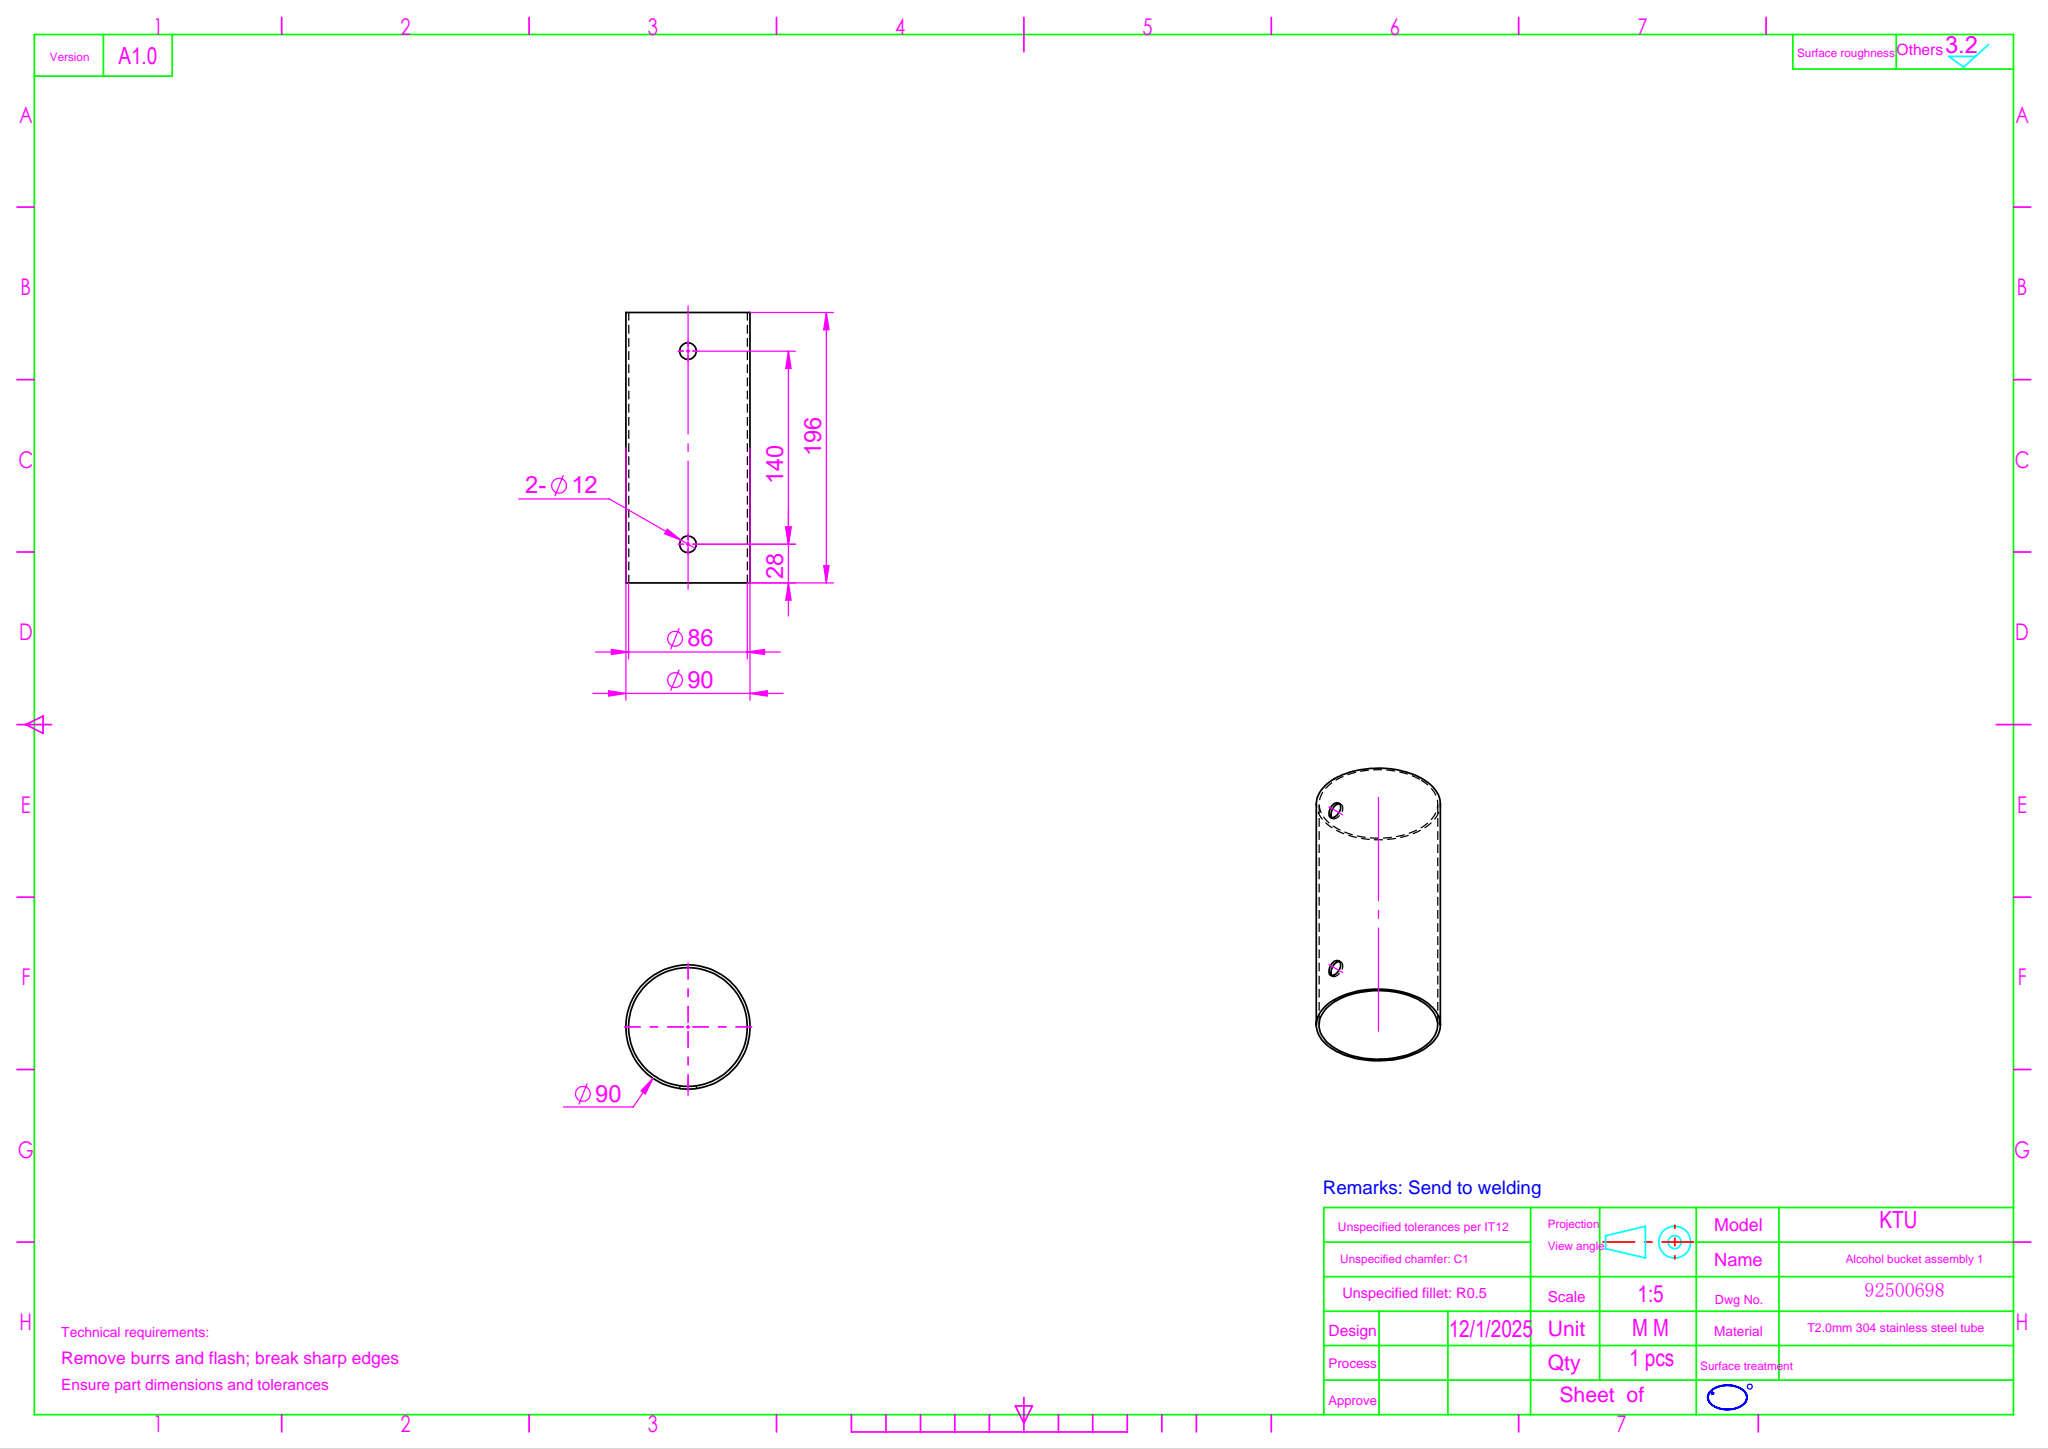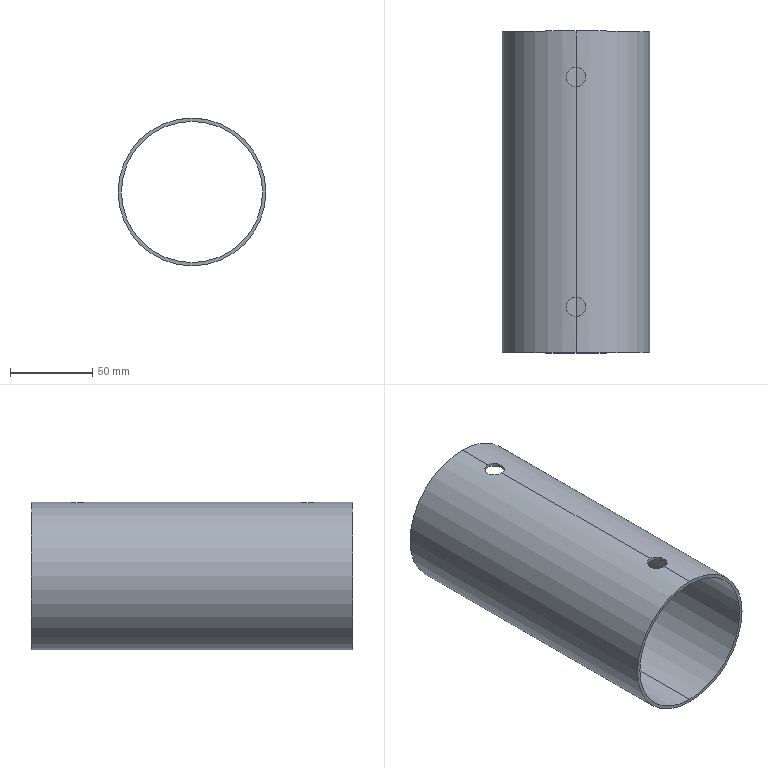Part | SolidWorks | features ExtruThin 1, ICE 1 | 1 solid | 10 faces | box 90 x 196 x 90 mm | volume 107919 mm3 | cylinder 8 | plane 2 | commonest cylinder face diameters 12 x4 86 x2 90 x2
STEP:
#1=CARTESIAN_POINT('',(0.,-76.,45.));
#2=VERTEX_POINT('',#1);
#3=CARTESIAN_POINT('',(6.,-70.,44.598));
#4=VERTEX_POINT('',#3);
#5=CARTESIAN_POINT('',(0.,-76.,45.));
#6=CARTESIAN_POINT('',(0.397,-76.,45.));
#7=CARTESIAN_POINT('',(0.7873,-75.961,44.995));
#8=CARTESIAN_POINT('',(1.363,-75.846,44.98));
#9=CARTESIAN_POINT('',(1.553,-75.799,44.974));
#10=CARTESIAN_POINT('',(1.931,-75.684,44.959));
#11=CARTESIAN_POINT('',(2.118,-75.617,44.95));
#12=CARTESIAN_POINT('',(2.663,-75.391,44.923));
#13=CARTESIAN_POINT('',(3.008,-75.207,44.901));
#14=CARTESIAN_POINT('',(3.66,-74.771,44.852));
#15=CARTESIAN_POINT('',(3.968,-74.518,44.826));
#16=CARTESIAN_POINT('',(4.521,-73.964,44.773));
#17=CARTESIAN_POINT('',(4.769,-73.662,44.747));
#18=CARTESIAN_POINT('',(5.098,-73.17,44.71));
#19=CARTESIAN_POINT('',(5.2,-73.,44.699));
#20=CARTESIAN_POINT('',(5.385,-72.654,44.677));
#21=CARTESIAN_POINT('',(5.552,-72.3,44.656));
#22=CARTESIAN_POINT('',(5.684,-71.932,44.64));
#23=CARTESIAN_POINT('',(5.798,-71.556,44.625));
#24=CARTESIAN_POINT('',(5.846,-71.363,44.619));
#25=CARTESIAN_POINT('',(5.962,-70.782,44.603));
#26=CARTESIAN_POINT('',(6.,-70.392,44.598));
#27=CARTESIAN_POINT('',(6.,-70.,44.598));
#28=B_SPLINE_CURVE_WITH_KNOTS('',3,(#5,#6,#7,#8,#9,#10,#11,#12,#13,#14,#15,#16,#17,#18,#19,#20,#21,#22,#23,#24,#25,#26,#27),.UNSPECIFIED.,.F.,.F.,(4,2,2,2,2,2,2,2,1,2,2,4),(0.,0.001174,0.001761,0.002348,0.003522,0.004696,0.00587,0.006457,0.007044,0.007631,0.008218,0.009392),.UNSPECIFIED.);
#29=EDGE_CURVE('',#2,#4,#28,.T.);
#30=ORIENTED_EDGE('',*,*,#29,.T.);
#31=CARTESIAN_POINT('',(6.,-70.,42.579));
#32=VERTEX_POINT('',#31);
#33=CARTESIAN_POINT('',(6.,-70.,45.));
#34=DIRECTION('',(0.,0.,-1.));
#35=VECTOR('',#34,1000.);
#36=LINE('',#33,#35);
#37=EDGE_CURVE('',#4,#32,#36,.T.);
#38=ORIENTED_EDGE('',*,*,#37,.T.);
#39=CARTESIAN_POINT('',(0.,-76.,43.));
#40=VERTEX_POINT('',#39);
#41=CARTESIAN_POINT('',(0.,-76.,43.));
#42=CARTESIAN_POINT('',(0.3918,-76.,43.));
#43=CARTESIAN_POINT('',(0.7898,-75.961,42.994));
#44=CARTESIAN_POINT('',(1.559,-75.807,42.973));
#45=CARTESIAN_POINT('',(1.934,-75.693,42.958));
#46=CARTESIAN_POINT('',(2.479,-75.468,42.929));
#47=CARTESIAN_POINT('',(2.659,-75.382,42.918));
#48=CARTESIAN_POINT('',(3.005,-75.197,42.895));
#49=CARTESIAN_POINT('',(3.173,-75.096,42.883));
#50=CARTESIAN_POINT('',(3.66,-74.77,42.845));
#51=CARTESIAN_POINT('',(3.964,-74.522,42.818));
#52=CARTESIAN_POINT('',(4.523,-73.962,42.762));
#53=CARTESIAN_POINT('',(4.771,-73.66,42.735));
#54=CARTESIAN_POINT('',(5.096,-73.173,42.697));
#55=CARTESIAN_POINT('',(5.197,-73.005,42.685));
#56=CARTESIAN_POINT('',(5.383,-72.658,42.662));
#57=CARTESIAN_POINT('',(5.468,-72.478,42.651));
#58=CARTESIAN_POINT('',(5.694,-71.933,42.622));
#59=CARTESIAN_POINT('',(5.807,-71.559,42.606));
#60=CARTESIAN_POINT('',(5.961,-70.79,42.585));
#61=CARTESIAN_POINT('',(6.,-70.392,42.579));
#62=CARTESIAN_POINT('',(6.,-70.,42.579));
#63=B_SPLINE_CURVE_WITH_KNOTS('',3,(#41,#42,#43,#44,#45,#46,#47,#48,#49,#50,#51,#52,#53,#54,#55,#56,#57,#58,#59,#60,#61,#62),.UNSPECIFIED.,.F.,.F.,(4,2,2,2,2,2,2,2,2,2,4),(0.009393,0.01057,0.01174,0.01233,0.01291,0.01409,0.01526,0.01585,0.01643,0.01761,0.01878),.UNSPECIFIED.);
#64=EDGE_CURVE('',#40,#32,#63,.T.);
#65=ORIENTED_EDGE('',*,*,#64,.F.);
#66=CARTESIAN_POINT('',(-6.,-70.,42.579));
#67=VERTEX_POINT('',#66);
#68=CARTESIAN_POINT('',(-6.,-70.,42.579));
#69=CARTESIAN_POINT('',(-6.,-70.397,42.579));
#70=CARTESIAN_POINT('',(-5.961,-70.787,42.585));
#71=CARTESIAN_POINT('',(-5.846,-71.363,42.601));
#72=CARTESIAN_POINT('',(-5.799,-71.553,42.607));
#73=CARTESIAN_POINT('',(-5.684,-71.931,42.623));
#74=CARTESIAN_POINT('',(-5.617,-72.118,42.632));
#75=CARTESIAN_POINT('',(-5.391,-72.663,42.661));
#76=CARTESIAN_POINT('',(-5.207,-73.008,42.684));
#77=CARTESIAN_POINT('',(-4.771,-73.66,42.735));
#78=CARTESIAN_POINT('',(-4.518,-73.968,42.763));
#79=CARTESIAN_POINT('',(-3.964,-74.521,42.818));
#80=CARTESIAN_POINT('',(-3.662,-74.769,42.845));
#81=CARTESIAN_POINT('',(-3.17,-75.098,42.883));
#82=CARTESIAN_POINT('',(-3.,-75.2,42.896));
#83=CARTESIAN_POINT('',(-2.654,-75.385,42.918));
#84=CARTESIAN_POINT('',(-2.3,-75.552,42.94));
#85=CARTESIAN_POINT('',(-1.932,-75.684,42.957));
#86=CARTESIAN_POINT('',(-1.556,-75.798,42.972));
#87=CARTESIAN_POINT('',(-1.363,-75.846,42.979));
#88=CARTESIAN_POINT('',(-0.7817,-75.962,42.995));
#89=CARTESIAN_POINT('',(-0.392,-76.,43.));
#90=CARTESIAN_POINT('',(0.,-76.,43.));
#91=B_SPLINE_CURVE_WITH_KNOTS('',3,(#68,#69,#70,#71,#72,#73,#74,#75,#76,#77,#78,#79,#80,#81,#82,#83,#84,#85,#86,#87,#88,#89,#90),.UNSPECIFIED.,.F.,.F.,(4,2,2,2,2,2,2,2,1,2,2,4),(0.,0.001174,0.001761,0.002348,0.003522,0.004697,0.005871,0.006458,0.007045,0.007632,0.008219,0.009393),.UNSPECIFIED.);
#92=EDGE_CURVE('',#67,#40,#91,.T.);
#93=ORIENTED_EDGE('',*,*,#92,.F.);
#94=CARTESIAN_POINT('',(-6.,-70.,44.598));
#95=VERTEX_POINT('',#94);
#96=CARTESIAN_POINT('',(-6.,-70.,45.));
#97=DIRECTION('',(0.,0.,-1.));
#98=VECTOR('',#97,1000.);
#99=LINE('',#96,#98);
#100=EDGE_CURVE('',#95,#67,#99,.T.);
#101=ORIENTED_EDGE('',*,*,#100,.F.);
#102=CARTESIAN_POINT('',(-6.,-70.,44.598));
#103=CARTESIAN_POINT('',(-6.,-70.396,44.598));
#104=CARTESIAN_POINT('',(-5.961,-70.786,44.603));
#105=CARTESIAN_POINT('',(-5.847,-71.362,44.619));
#106=CARTESIAN_POINT('',(-5.799,-71.552,44.625));
#107=CARTESIAN_POINT('',(-5.685,-71.929,44.64));
#108=CARTESIAN_POINT('',(-5.618,-72.116,44.648));
#109=CARTESIAN_POINT('',(-5.392,-72.661,44.676));
#110=CARTESIAN_POINT('',(-5.208,-73.005,44.698));
#111=CARTESIAN_POINT('',(-4.773,-73.657,44.747));
#112=CARTESIAN_POINT('',(-4.52,-73.965,44.773));
#113=CARTESIAN_POINT('',(-3.968,-74.517,44.826));
#114=CARTESIAN_POINT('',(-3.666,-74.766,44.852));
#115=CARTESIAN_POINT('',(-3.011,-75.205,44.9));
#116=CARTESIAN_POINT('',(-2.663,-75.391,44.923));
#117=CARTESIAN_POINT('',(-1.942,-75.69,44.96));
#118=CARTESIAN_POINT('',(-1.564,-75.806,44.974));
#119=CARTESIAN_POINT('',(-0.7887,-75.961,44.995));
#120=CARTESIAN_POINT('',(-0.3966,-76.,45.));
#121=CARTESIAN_POINT('',(0.,-76.,45.));
#122=B_SPLINE_CURVE_WITH_KNOTS('',3,(#102,#103,#104,#105,#106,#107,#108,#109,#110,#111,#112,#113,#114,#115,#116,#117,#118,#119,#120,#121),.UNSPECIFIED.,.F.,.F.,(4,2,2,2,2,2,2,2,2,4),(0.02817,0.02934,0.02993,0.03052,0.03169,0.03286,0.03404,0.03521,0.03638,0.03755),.UNSPECIFIED.);
#123=EDGE_CURVE('',#95,#2,#122,.T.);
#124=ORIENTED_EDGE('',*,*,#123,.T.);
#125=EDGE_LOOP('',(#30,#38,#65,#93,#101,#124));
#126=FACE_OUTER_BOUND('',#125,.T.);
#127=CARTESIAN_POINT('',(0.,-70.,45.));
#128=DIRECTION('',(0.,0.,-1.));
#129=DIRECTION('',(-1.,0.,0.));
#130=AXIS2_PLACEMENT_3D('',#127,#128,#129);
#131=CYLINDRICAL_SURFACE('',#130,6.);
#132=ADVANCED_FACE('',(#126),#131,.F.);
#133=CARTESIAN_POINT('',(0.,64.,45.));
#134=VERTEX_POINT('',#133);
#135=CARTESIAN_POINT('',(6.,70.,44.598));
#136=VERTEX_POINT('',#135);
#137=CARTESIAN_POINT('',(0.,64.,45.));
#138=CARTESIAN_POINT('',(0.397,64.,45.));
#139=CARTESIAN_POINT('',(0.7873,64.039,44.995));
#140=CARTESIAN_POINT('',(1.363,64.154,44.98));
#141=CARTESIAN_POINT('',(1.553,64.201,44.974));
#142=CARTESIAN_POINT('',(1.931,64.316,44.959));
#143=CARTESIAN_POINT('',(2.118,64.383,44.95));
#144=CARTESIAN_POINT('',(2.663,64.609,44.923));
#145=CARTESIAN_POINT('',(3.008,64.793,44.901));
#146=CARTESIAN_POINT('',(3.66,65.229,44.852));
#147=CARTESIAN_POINT('',(3.968,65.482,44.826));
#148=CARTESIAN_POINT('',(4.521,66.036,44.773));
#149=CARTESIAN_POINT('',(4.769,66.338,44.747));
#150=CARTESIAN_POINT('',(5.098,66.83,44.71));
#151=CARTESIAN_POINT('',(5.2,67.,44.699));
#152=CARTESIAN_POINT('',(5.385,67.346,44.677));
#153=CARTESIAN_POINT('',(5.552,67.7,44.656));
#154=CARTESIAN_POINT('',(5.684,68.068,44.64));
#155=CARTESIAN_POINT('',(5.798,68.444,44.625));
#156=CARTESIAN_POINT('',(5.846,68.637,44.619));
#157=CARTESIAN_POINT('',(5.962,69.218,44.603));
#158=CARTESIAN_POINT('',(6.,69.608,44.598));
#159=CARTESIAN_POINT('',(6.,70.,44.598));
#160=B_SPLINE_CURVE_WITH_KNOTS('',3,(#137,#138,#139,#140,#141,#142,#143,#144,#145,#146,#147,#148,#149,#150,#151,#152,#153,#154,#155,#156,#157,#158,#159),.UNSPECIFIED.,.F.,.F.,(4,2,2,2,2,2,2,2,1,2,2,4),(0.,0.001174,0.001761,0.002348,0.003522,0.004696,0.00587,0.006457,0.007044,0.007631,0.008218,0.009392),.UNSPECIFIED.);
#161=EDGE_CURVE('',#134,#136,#160,.T.);
#162=ORIENTED_EDGE('',*,*,#161,.T.);
#163=CARTESIAN_POINT('',(6.,70.,42.579));
#164=VERTEX_POINT('',#163);
#165=CARTESIAN_POINT('',(6.,70.,45.));
#166=DIRECTION('',(0.,0.,-1.));
#167=VECTOR('',#166,1000.);
#168=LINE('',#165,#167);
#169=EDGE_CURVE('',#136,#164,#168,.T.);
#170=ORIENTED_EDGE('',*,*,#169,.T.);
#171=CARTESIAN_POINT('',(0.,64.,43.));
#172=VERTEX_POINT('',#171);
#173=CARTESIAN_POINT('',(0.,64.,43.));
#174=CARTESIAN_POINT('',(0.3918,64.,43.));
#175=CARTESIAN_POINT('',(0.7898,64.039,42.994));
#176=CARTESIAN_POINT('',(1.559,64.193,42.973));
#177=CARTESIAN_POINT('',(1.934,64.307,42.958));
#178=CARTESIAN_POINT('',(2.479,64.532,42.929));
#179=CARTESIAN_POINT('',(2.659,64.618,42.918));
#180=CARTESIAN_POINT('',(3.005,64.803,42.895));
#181=CARTESIAN_POINT('',(3.173,64.904,42.883));
#182=CARTESIAN_POINT('',(3.66,65.23,42.845));
#183=CARTESIAN_POINT('',(3.964,65.478,42.818));
#184=CARTESIAN_POINT('',(4.523,66.038,42.762));
#185=CARTESIAN_POINT('',(4.771,66.34,42.735));
#186=CARTESIAN_POINT('',(5.096,66.827,42.697));
#187=CARTESIAN_POINT('',(5.197,66.995,42.685));
#188=CARTESIAN_POINT('',(5.383,67.342,42.662));
#189=CARTESIAN_POINT('',(5.468,67.522,42.651));
#190=CARTESIAN_POINT('',(5.694,68.067,42.622));
#191=CARTESIAN_POINT('',(5.807,68.441,42.606));
#192=CARTESIAN_POINT('',(5.961,69.21,42.585));
#193=CARTESIAN_POINT('',(6.,69.608,42.579));
#194=CARTESIAN_POINT('',(6.,70.,42.579));
#195=B_SPLINE_CURVE_WITH_KNOTS('',3,(#173,#174,#175,#176,#177,#178,#179,#180,#181,#182,#183,#184,#185,#186,#187,#188,#189,#190,#191,#192,#193,#194),.UNSPECIFIED.,.F.,.F.,(4,2,2,2,2,2,2,2,2,2,4),(0.009393,0.01057,0.01174,0.01233,0.01291,0.01409,0.01526,0.01585,0.01643,0.01761,0.01878),.UNSPECIFIED.);
#196=EDGE_CURVE('',#172,#164,#195,.T.);
#197=ORIENTED_EDGE('',*,*,#196,.F.);
#198=CARTESIAN_POINT('',(-6.,70.,42.579));
#199=VERTEX_POINT('',#198);
#200=CARTESIAN_POINT('',(-6.,70.,42.579));
#201=CARTESIAN_POINT('',(-6.,69.603,42.579));
#202=CARTESIAN_POINT('',(-5.961,69.213,42.585));
#203=CARTESIAN_POINT('',(-5.846,68.637,42.601));
#204=CARTESIAN_POINT('',(-5.799,68.447,42.607));
#205=CARTESIAN_POINT('',(-5.684,68.069,42.623));
#206=CARTESIAN_POINT('',(-5.617,67.882,42.632));
#207=CARTESIAN_POINT('',(-5.391,67.337,42.661));
#208=CARTESIAN_POINT('',(-5.207,66.992,42.684));
#209=CARTESIAN_POINT('',(-4.771,66.34,42.735));
#210=CARTESIAN_POINT('',(-4.518,66.032,42.763));
#211=CARTESIAN_POINT('',(-3.964,65.479,42.818));
#212=CARTESIAN_POINT('',(-3.662,65.231,42.845));
#213=CARTESIAN_POINT('',(-3.17,64.902,42.883));
#214=CARTESIAN_POINT('',(-3.,64.8,42.896));
#215=CARTESIAN_POINT('',(-2.654,64.615,42.918));
#216=CARTESIAN_POINT('',(-2.3,64.448,42.94));
#217=CARTESIAN_POINT('',(-1.932,64.316,42.957));
#218=CARTESIAN_POINT('',(-1.556,64.202,42.972));
#219=CARTESIAN_POINT('',(-1.363,64.154,42.979));
#220=CARTESIAN_POINT('',(-0.7817,64.038,42.995));
#221=CARTESIAN_POINT('',(-0.392,64.,43.));
#222=CARTESIAN_POINT('',(0.,64.,43.));
#223=B_SPLINE_CURVE_WITH_KNOTS('',3,(#200,#201,#202,#203,#204,#205,#206,#207,#208,#209,#210,#211,#212,#213,#214,#215,#216,#217,#218,#219,#220,#221,#222),.UNSPECIFIED.,.F.,.F.,(4,2,2,2,2,2,2,2,1,2,2,4),(0.,0.001174,0.001761,0.002348,0.003522,0.004697,0.005871,0.006458,0.007045,0.007632,0.008219,0.009393),.UNSPECIFIED.);
#224=EDGE_CURVE('',#199,#172,#223,.T.);
#225=ORIENTED_EDGE('',*,*,#224,.F.);
#226=CARTESIAN_POINT('',(-6.,70.,44.598));
#227=VERTEX_POINT('',#226);
#228=CARTESIAN_POINT('',(-6.,70.,45.));
#229=DIRECTION('',(0.,0.,-1.));
#230=VECTOR('',#229,1000.);
#231=LINE('',#228,#230);
#232=EDGE_CURVE('',#227,#199,#231,.T.);
#233=ORIENTED_EDGE('',*,*,#232,.F.);
#234=CARTESIAN_POINT('',(-6.,70.,44.598));
#235=CARTESIAN_POINT('',(-6.,69.604,44.598));
#236=CARTESIAN_POINT('',(-5.961,69.214,44.603));
#237=CARTESIAN_POINT('',(-5.847,68.638,44.619));
#238=CARTESIAN_POINT('',(-5.799,68.448,44.625));
#239=CARTESIAN_POINT('',(-5.685,68.071,44.64));
#240=CARTESIAN_POINT('',(-5.618,67.884,44.648));
#241=CARTESIAN_POINT('',(-5.392,67.339,44.676));
#242=CARTESIAN_POINT('',(-5.208,66.995,44.698));
#243=CARTESIAN_POINT('',(-4.773,66.343,44.747));
#244=CARTESIAN_POINT('',(-4.52,66.035,44.773));
#245=CARTESIAN_POINT('',(-3.968,65.483,44.826));
#246=CARTESIAN_POINT('',(-3.666,65.234,44.852));
#247=CARTESIAN_POINT('',(-3.011,64.795,44.9));
#248=CARTESIAN_POINT('',(-2.663,64.609,44.923));
#249=CARTESIAN_POINT('',(-1.942,64.31,44.96));
#250=CARTESIAN_POINT('',(-1.564,64.194,44.974));
#251=CARTESIAN_POINT('',(-0.7887,64.039,44.995));
#252=CARTESIAN_POINT('',(-0.3966,64.,45.));
#253=CARTESIAN_POINT('',(0.,64.,45.));
#254=B_SPLINE_CURVE_WITH_KNOTS('',3,(#234,#235,#236,#237,#238,#239,#240,#241,#242,#243,#244,#245,#246,#247,#248,#249,#250,#251,#252,#253),.UNSPECIFIED.,.F.,.F.,(4,2,2,2,2,2,2,2,2,4),(0.02817,0.02934,0.02993,0.03052,0.03169,0.03286,0.03404,0.03521,0.03638,0.03755),.UNSPECIFIED.);
#255=EDGE_CURVE('',#227,#134,#254,.T.);
#256=ORIENTED_EDGE('',*,*,#255,.T.);
#257=EDGE_LOOP('',(#162,#170,#197,#225,#233,#256));
#258=FACE_OUTER_BOUND('',#257,.T.);
#259=CARTESIAN_POINT('',(0.,70.,45.));
#260=DIRECTION('',(0.,0.,-1.));
#261=DIRECTION('',(-1.,0.,0.));
#262=AXIS2_PLACEMENT_3D('',#259,#260,#261);
#263=CYLINDRICAL_SURFACE('',#262,6.);
#264=ADVANCED_FACE('',(#258),#263,.F.);
#265=CARTESIAN_POINT('',(0.,98.,-43.));
#266=VERTEX_POINT('',#265);
#267=CARTESIAN_POINT('',(0.,98.,43.));
#268=VERTEX_POINT('',#267);
#269=CARTESIAN_POINT('',(0.,98.,0.));
#270=DIRECTION('',(0.,1.,0.));
#271=DIRECTION('',(1.,0.,0.));
#272=AXIS2_PLACEMENT_3D('',#269,#270,#271);
#273=CIRCLE('',#272,43.);
#274=EDGE_CURVE('',#266,#268,#273,.T.);
#275=ORIENTED_EDGE('',*,*,#274,.T.);
#276=CARTESIAN_POINT('',(0.,76.,43.));
#277=VERTEX_POINT('',#276);
#278=CARTESIAN_POINT('',(0.,98.,43.));
#279=DIRECTION('',(0.,-1.,0.));
#280=VECTOR('',#279,1000.);
#281=LINE('',#278,#280);
#282=EDGE_CURVE('',#268,#277,#281,.T.);
#283=ORIENTED_EDGE('',*,*,#282,.T.);
#284=CARTESIAN_POINT('',(0.,76.,43.));
#285=CARTESIAN_POINT('',(-0.3964,76.,43.));
#286=CARTESIAN_POINT('',(-0.7863,75.961,42.995));
#287=CARTESIAN_POINT('',(-1.362,75.847,42.979));
#288=CARTESIAN_POINT('',(-1.552,75.799,42.972));
#289=CARTESIAN_POINT('',(-1.929,75.685,42.957));
#290=CARTESIAN_POINT('',(-2.116,75.618,42.948));
#291=CARTESIAN_POINT('',(-2.661,75.392,42.919));
#292=CARTESIAN_POINT('',(-3.005,75.208,42.896));
#293=CARTESIAN_POINT('',(-3.657,74.773,42.845));
#294=CARTESIAN_POINT('',(-3.965,74.52,42.818));
#295=CARTESIAN_POINT('',(-4.517,73.968,42.763));
#296=CARTESIAN_POINT('',(-4.766,73.667,42.736));
#297=CARTESIAN_POINT('',(-5.205,73.011,42.684));
#298=CARTESIAN_POINT('',(-5.391,72.663,42.661));
#299=CARTESIAN_POINT('',(-5.69,71.942,42.622));
#300=CARTESIAN_POINT('',(-5.806,71.564,42.606));
#301=CARTESIAN_POINT('',(-5.961,70.789,42.585));
#302=CARTESIAN_POINT('',(-6.,70.397,42.579));
#303=CARTESIAN_POINT('',(-6.,70.,42.579));
#304=B_SPLINE_CURVE_WITH_KNOTS('',3,(#284,#285,#286,#287,#288,#289,#290,#291,#292,#293,#294,#295,#296,#297,#298,#299,#300,#301,#302,#303),.UNSPECIFIED.,.F.,.F.,(4,2,2,2,2,2,2,2,2,4),(0.02817,0.02935,0.02993,0.03052,0.03169,0.03287,0.03404,0.03521,0.03639,0.03756),.UNSPECIFIED.);
#305=EDGE_CURVE('',#277,#199,#304,.T.);
#306=ORIENTED_EDGE('',*,*,#305,.T.);
#307=ORIENTED_EDGE('',*,*,#224,.T.);
#308=CARTESIAN_POINT('',(0.,-64.,43.));
#309=VERTEX_POINT('',#308);
#310=CARTESIAN_POINT('',(0.,98.,43.));
#311=DIRECTION('',(0.,-1.,0.));
#312=VECTOR('',#311,1000.);
#313=LINE('',#310,#312);
#314=EDGE_CURVE('',#172,#309,#313,.T.);
#315=ORIENTED_EDGE('',*,*,#314,.T.);
#316=CARTESIAN_POINT('',(0.,-64.,43.));
#317=CARTESIAN_POINT('',(-0.3964,-64.,43.));
#318=CARTESIAN_POINT('',(-0.7863,-64.039,42.995));
#319=CARTESIAN_POINT('',(-1.362,-64.153,42.979));
#320=CARTESIAN_POINT('',(-1.552,-64.201,42.972));
#321=CARTESIAN_POINT('',(-1.929,-64.315,42.957));
#322=CARTESIAN_POINT('',(-2.116,-64.382,42.948));
#323=CARTESIAN_POINT('',(-2.661,-64.608,42.919));
#324=CARTESIAN_POINT('',(-3.005,-64.792,42.896));
#325=CARTESIAN_POINT('',(-3.657,-65.227,42.845));
#326=CARTESIAN_POINT('',(-3.965,-65.48,42.818));
#327=CARTESIAN_POINT('',(-4.517,-66.032,42.763));
#328=CARTESIAN_POINT('',(-4.766,-66.333,42.736));
#329=CARTESIAN_POINT('',(-5.205,-66.989,42.684));
#330=CARTESIAN_POINT('',(-5.391,-67.337,42.661));
#331=CARTESIAN_POINT('',(-5.69,-68.058,42.622));
#332=CARTESIAN_POINT('',(-5.806,-68.436,42.606));
#333=CARTESIAN_POINT('',(-5.961,-69.211,42.585));
#334=CARTESIAN_POINT('',(-6.,-69.603,42.579));
#335=CARTESIAN_POINT('',(-6.,-70.,42.579));
#336=B_SPLINE_CURVE_WITH_KNOTS('',3,(#316,#317,#318,#319,#320,#321,#322,#323,#324,#325,#326,#327,#328,#329,#330,#331,#332,#333,#334,#335),.UNSPECIFIED.,.F.,.F.,(4,2,2,2,2,2,2,2,2,4),(0.02817,0.02935,0.02993,0.03052,0.03169,0.03287,0.03404,0.03521,0.03639,0.03756),.UNSPECIFIED.);
#337=EDGE_CURVE('',#309,#67,#336,.T.);
#338=ORIENTED_EDGE('',*,*,#337,.T.);
#339=ORIENTED_EDGE('',*,*,#92,.T.);
#340=CARTESIAN_POINT('',(0.,-98.,43.));
#341=VERTEX_POINT('',#340);
#342=CARTESIAN_POINT('',(0.,98.,43.));
#343=DIRECTION('',(0.,-1.,0.));
#344=VECTOR('',#343,1000.);
#345=LINE('',#342,#344);
#346=EDGE_CURVE('',#40,#341,#345,.T.);
#347=ORIENTED_EDGE('',*,*,#346,.T.);
#348=CARTESIAN_POINT('',(0.,-98.,-43.));
#349=VERTEX_POINT('',#348);
#350=CARTESIAN_POINT('',(0.,-98.,0.));
#351=DIRECTION('',(0.,1.,0.));
#352=DIRECTION('',(1.,0.,0.));
#353=AXIS2_PLACEMENT_3D('',#350,#351,#352);
#354=CIRCLE('',#353,43.);
#355=EDGE_CURVE('',#349,#341,#354,.T.);
#356=ORIENTED_EDGE('',*,*,#355,.F.);
#357=CARTESIAN_POINT('',(0.,98.,-43.));
#358=DIRECTION('',(0.,-1.,0.));
#359=VECTOR('',#358,1000.);
#360=LINE('',#357,#359);
#361=EDGE_CURVE('',#266,#349,#360,.T.);
#362=ORIENTED_EDGE('',*,*,#361,.F.);
#363=EDGE_LOOP('',(#275,#283,#306,#307,#315,#338,#339,#347,#356,#362));
#364=FACE_OUTER_BOUND('',#363,.T.);
#365=CARTESIAN_POINT('',(0.,98.,0.));
#366=DIRECTION('',(0.,-1.,0.));
#367=DIRECTION('',(0.,0.,-1.));
#368=AXIS2_PLACEMENT_3D('',#365,#366,#367);
#369=CYLINDRICAL_SURFACE('',#368,43.);
#370=ADVANCED_FACE('',(#364),#369,.F.);
#371=CARTESIAN_POINT('',(0.,98.,45.));
#372=VERTEX_POINT('',#371);
#373=CARTESIAN_POINT('',(0.,98.,-45.));
#374=VERTEX_POINT('',#373);
#375=CARTESIAN_POINT('',(0.,98.,0.));
#376=DIRECTION('',(0.,1.,0.));
#377=DIRECTION('',(0.,0.,1.));
#378=AXIS2_PLACEMENT_3D('',#375,#376,#377);
#379=CIRCLE('',#378,45.);
#380=EDGE_CURVE('',#372,#374,#379,.T.);
#381=ORIENTED_EDGE('',*,*,#380,.F.);
#382=CARTESIAN_POINT('',(0.,76.,45.));
#383=VERTEX_POINT('',#382);
#384=CARTESIAN_POINT('',(0.,98.,45.));
#385=DIRECTION('',(0.,-1.,0.));
#386=VECTOR('',#385,1000.);
#387=LINE('',#384,#386);
#388=EDGE_CURVE('',#372,#383,#387,.T.);
#389=ORIENTED_EDGE('',*,*,#388,.T.);
#390=CARTESIAN_POINT('',(6.,70.,44.598));
#391=CARTESIAN_POINT('',(6.,70.392,44.598));
#392=CARTESIAN_POINT('',(5.961,70.79,44.604));
#393=CARTESIAN_POINT('',(5.807,71.559,44.624));
#394=CARTESIAN_POINT('',(5.694,71.933,44.639));
#395=CARTESIAN_POINT('',(5.468,72.479,44.667));
#396=CARTESIAN_POINT('',(5.383,72.658,44.677));
#397=CARTESIAN_POINT('',(5.197,73.005,44.699));
#398=CARTESIAN_POINT('',(5.096,73.173,44.711));
#399=CARTESIAN_POINT('',(4.77,73.66,44.747));
#400=CARTESIAN_POINT('',(4.522,73.963,44.773));
#401=CARTESIAN_POINT('',(3.962,74.523,44.826));
#402=CARTESIAN_POINT('',(3.66,74.771,44.852));
#403=CARTESIAN_POINT('',(3.173,75.096,44.888));
#404=CARTESIAN_POINT('',(3.005,75.197,44.9));
#405=CARTESIAN_POINT('',(2.658,75.383,44.922));
#406=CARTESIAN_POINT('',(2.478,75.468,44.932));
#407=CARTESIAN_POINT('',(1.933,75.694,44.96));
#408=CARTESIAN_POINT('',(1.559,75.807,44.975));
#409=CARTESIAN_POINT('',(0.7896,75.961,44.995));
#410=CARTESIAN_POINT('',(0.3917,76.,45.));
#411=CARTESIAN_POINT('',(0.,76.,45.));
#412=B_SPLINE_CURVE_WITH_KNOTS('',3,(#390,#391,#392,#393,#394,#395,#396,#397,#398,#399,#400,#401,#402,#403,#404,#405,#406,#407,#408,#409,#410,#411),.UNSPECIFIED.,.F.,.F.,(4,2,2,2,2,2,2,2,2,2,4),(0.009392,0.01057,0.01174,0.01233,0.01291,0.01409,0.01526,0.01585,0.01643,0.01761,0.01878),.UNSPECIFIED.);
#413=EDGE_CURVE('',#136,#383,#412,.T.);
#414=ORIENTED_EDGE('',*,*,#413,.F.);
#415=ORIENTED_EDGE('',*,*,#161,.F.);
#416=CARTESIAN_POINT('',(0.,-64.,45.));
#417=VERTEX_POINT('',#416);
#418=CARTESIAN_POINT('',(0.,98.,45.));
#419=DIRECTION('',(0.,-1.,0.));
#420=VECTOR('',#419,1000.);
#421=LINE('',#418,#420);
#422=EDGE_CURVE('',#134,#417,#421,.T.);
#423=ORIENTED_EDGE('',*,*,#422,.T.);
#424=CARTESIAN_POINT('',(6.,-70.,44.598));
#425=CARTESIAN_POINT('',(6.,-69.608,44.598));
#426=CARTESIAN_POINT('',(5.961,-69.21,44.604));
#427=CARTESIAN_POINT('',(5.807,-68.441,44.624));
#428=CARTESIAN_POINT('',(5.694,-68.067,44.639));
#429=CARTESIAN_POINT('',(5.468,-67.521,44.667));
#430=CARTESIAN_POINT('',(5.383,-67.342,44.677));
#431=CARTESIAN_POINT('',(5.197,-66.995,44.699));
#432=CARTESIAN_POINT('',(5.096,-66.827,44.711));
#433=CARTESIAN_POINT('',(4.77,-66.34,44.747));
#434=CARTESIAN_POINT('',(4.522,-66.037,44.773));
#435=CARTESIAN_POINT('',(3.962,-65.477,44.826));
#436=CARTESIAN_POINT('',(3.66,-65.229,44.852));
#437=CARTESIAN_POINT('',(3.173,-64.904,44.888));
#438=CARTESIAN_POINT('',(3.005,-64.803,44.9));
#439=CARTESIAN_POINT('',(2.658,-64.617,44.922));
#440=CARTESIAN_POINT('',(2.478,-64.532,44.932));
#441=CARTESIAN_POINT('',(1.933,-64.306,44.96));
#442=CARTESIAN_POINT('',(1.559,-64.193,44.975));
#443=CARTESIAN_POINT('',(0.7896,-64.039,44.995));
#444=CARTESIAN_POINT('',(0.3917,-64.,45.));
#445=CARTESIAN_POINT('',(0.,-64.,45.));
#446=B_SPLINE_CURVE_WITH_KNOTS('',3,(#424,#425,#426,#427,#428,#429,#430,#431,#432,#433,#434,#435,#436,#437,#438,#439,#440,#441,#442,#443,#444,#445),.UNSPECIFIED.,.F.,.F.,(4,2,2,2,2,2,2,2,2,2,4),(0.009392,0.01057,0.01174,0.01233,0.01291,0.01409,0.01526,0.01585,0.01643,0.01761,0.01878),.UNSPECIFIED.);
#447=EDGE_CURVE('',#4,#417,#446,.T.);
#448=ORIENTED_EDGE('',*,*,#447,.F.);
#449=ORIENTED_EDGE('',*,*,#29,.F.);
#450=CARTESIAN_POINT('',(0.,-98.,45.));
#451=VERTEX_POINT('',#450);
#452=CARTESIAN_POINT('',(0.,98.,45.));
#453=DIRECTION('',(0.,-1.,0.));
#454=VECTOR('',#453,1000.);
#455=LINE('',#452,#454);
#456=EDGE_CURVE('',#2,#451,#455,.T.);
#457=ORIENTED_EDGE('',*,*,#456,.T.);
#458=CARTESIAN_POINT('',(0.,-98.,-45.));
#459=VERTEX_POINT('',#458);
#460=CARTESIAN_POINT('',(0.,-98.,0.));
#461=DIRECTION('',(0.,1.,0.));
#462=DIRECTION('',(0.,0.,1.));
#463=AXIS2_PLACEMENT_3D('',#460,#461,#462);
#464=CIRCLE('',#463,45.);
#465=EDGE_CURVE('',#451,#459,#464,.T.);
#466=ORIENTED_EDGE('',*,*,#465,.T.);
#467=CARTESIAN_POINT('',(0.,98.,-45.));
#468=DIRECTION('',(0.,-1.,0.));
#469=VECTOR('',#468,1000.);
#470=LINE('',#467,#469);
#471=EDGE_CURVE('',#374,#459,#470,.T.);
#472=ORIENTED_EDGE('',*,*,#471,.F.);
#473=EDGE_LOOP('',(#381,#389,#414,#415,#423,#448,#449,#457,#466,#472));
#474=FACE_OUTER_BOUND('',#473,.T.);
#475=CARTESIAN_POINT('',(0.,98.,0.));
#476=DIRECTION('',(0.,-1.,0.));
#477=DIRECTION('',(0.,0.,-1.));
#478=AXIS2_PLACEMENT_3D('',#475,#476,#477);
#479=CYLINDRICAL_SURFACE('',#478,45.);
#480=ADVANCED_FACE('',(#474),#479,.T.);
#481=ORIENTED_EDGE('',*,*,#388,.F.);
#482=CARTESIAN_POINT('',(0.,98.,0.));
#483=DIRECTION('',(0.,1.,0.));
#484=DIRECTION('',(0.,0.,1.));
#485=AXIS2_PLACEMENT_3D('',#482,#483,#484);
#486=CIRCLE('',#485,45.);
#487=EDGE_CURVE('',#374,#372,#486,.T.);
#488=ORIENTED_EDGE('',*,*,#487,.F.);
#489=ORIENTED_EDGE('',*,*,#471,.T.);
#490=CARTESIAN_POINT('',(0.,-98.,0.));
#491=DIRECTION('',(0.,1.,0.));
#492=DIRECTION('',(0.,0.,1.));
#493=AXIS2_PLACEMENT_3D('',#490,#491,#492);
#494=CIRCLE('',#493,45.);
#495=EDGE_CURVE('',#459,#451,#494,.T.);
#496=ORIENTED_EDGE('',*,*,#495,.T.);
#497=ORIENTED_EDGE('',*,*,#456,.F.);
#498=ORIENTED_EDGE('',*,*,#123,.F.);
#499=CARTESIAN_POINT('',(0.,-64.,45.));
#500=CARTESIAN_POINT('',(-0.3919,-64.,45.));
#501=CARTESIAN_POINT('',(-0.7817,-64.038,44.995));
#502=CARTESIAN_POINT('',(-1.363,-64.154,44.98));
#503=CARTESIAN_POINT('',(-1.556,-64.202,44.973));
#504=CARTESIAN_POINT('',(-1.932,-64.316,44.959));
#505=CARTESIAN_POINT('',(-2.3,-64.448,44.942));
#506=CARTESIAN_POINT('',(-2.654,-64.615,44.922));
#507=CARTESIAN_POINT('',(-3.001,-64.801,44.9));
#508=CARTESIAN_POINT('',(-3.171,-64.903,44.888));
#509=CARTESIAN_POINT('',(-3.663,-65.231,44.852));
#510=CARTESIAN_POINT('',(-3.965,-65.479,44.826));
#511=CARTESIAN_POINT('',(-4.518,-66.033,44.773));
#512=CARTESIAN_POINT('',(-4.771,-66.341,44.747));
#513=CARTESIAN_POINT('',(-5.207,-66.993,44.698));
#514=CARTESIAN_POINT('',(-5.391,-67.337,44.676));
#515=CARTESIAN_POINT('',(-5.617,-67.882,44.648));
#516=CARTESIAN_POINT('',(-5.684,-68.07,44.64));
#517=CARTESIAN_POINT('',(-5.799,-68.447,44.625));
#518=CARTESIAN_POINT('',(-5.846,-68.637,44.619));
#519=CARTESIAN_POINT('',(-5.961,-69.212,44.604));
#520=CARTESIAN_POINT('',(-6.,-69.603,44.598));
#521=CARTESIAN_POINT('',(-6.,-70.,44.598));
#522=B_SPLINE_CURVE_WITH_KNOTS('',3,(#499,#500,#501,#502,#503,#504,#505,#506,#507,#508,#509,#510,#511,#512,#513,#514,#515,#516,#517,#518,#519,#520,#521),.UNSPECIFIED.,.F.,.F.,(4,2,2,1,2,2,2,2,2,2,2,4),(0.01878,0.01995,0.02054,0.02113,0.02171,0.0223,0.02348,0.02465,0.02582,0.02641,0.027,0.02817),.UNSPECIFIED.);
#523=EDGE_CURVE('',#417,#95,#522,.T.);
#524=ORIENTED_EDGE('',*,*,#523,.F.);
#525=ORIENTED_EDGE('',*,*,#422,.F.);
#526=ORIENTED_EDGE('',*,*,#255,.F.);
#527=CARTESIAN_POINT('',(0.,76.,45.));
#528=CARTESIAN_POINT('',(-0.3919,76.,45.));
#529=CARTESIAN_POINT('',(-0.7817,75.962,44.995));
#530=CARTESIAN_POINT('',(-1.363,75.846,44.98));
#531=CARTESIAN_POINT('',(-1.556,75.798,44.973));
#532=CARTESIAN_POINT('',(-1.932,75.684,44.959));
#533=CARTESIAN_POINT('',(-2.3,75.552,44.942));
#534=CARTESIAN_POINT('',(-2.654,75.385,44.922));
#535=CARTESIAN_POINT('',(-3.001,75.199,44.9));
#536=CARTESIAN_POINT('',(-3.171,75.097,44.888));
#537=CARTESIAN_POINT('',(-3.663,74.769,44.852));
#538=CARTESIAN_POINT('',(-3.965,74.521,44.826));
#539=CARTESIAN_POINT('',(-4.518,73.967,44.773));
#540=CARTESIAN_POINT('',(-4.771,73.659,44.747));
#541=CARTESIAN_POINT('',(-5.207,73.007,44.698));
#542=CARTESIAN_POINT('',(-5.391,72.663,44.676));
#543=CARTESIAN_POINT('',(-5.617,72.118,44.648));
#544=CARTESIAN_POINT('',(-5.684,71.93,44.64));
#545=CARTESIAN_POINT('',(-5.799,71.553,44.625));
#546=CARTESIAN_POINT('',(-5.846,71.363,44.619));
#547=CARTESIAN_POINT('',(-5.961,70.788,44.604));
#548=CARTESIAN_POINT('',(-6.,70.397,44.598));
#549=CARTESIAN_POINT('',(-6.,70.,44.598));
#550=B_SPLINE_CURVE_WITH_KNOTS('',3,(#527,#528,#529,#530,#531,#532,#533,#534,#535,#536,#537,#538,#539,#540,#541,#542,#543,#544,#545,#546,#547,#548,#549),.UNSPECIFIED.,.F.,.F.,(4,2,2,1,2,2,2,2,2,2,2,4),(0.01878,0.01995,0.02054,0.02113,0.02171,0.0223,0.02348,0.02465,0.02582,0.02641,0.027,0.02817),.UNSPECIFIED.);
#551=EDGE_CURVE('',#383,#227,#550,.T.);
#552=ORIENTED_EDGE('',*,*,#551,.F.);
#553=EDGE_LOOP('',(#481,#488,#489,#496,#497,#498,#524,#525,#526,#552));
#554=FACE_OUTER_BOUND('',#553,.T.);
#555=CARTESIAN_POINT('',(0.,98.,0.));
#556=DIRECTION('',(0.,-1.,0.));
#557=DIRECTION('',(0.,0.,-1.));
#558=AXIS2_PLACEMENT_3D('',#555,#556,#557);
#559=CYLINDRICAL_SURFACE('',#558,45.);
#560=ADVANCED_FACE('',(#554),#559,.T.);
#561=ORIENTED_EDGE('',*,*,#282,.F.);
#562=CARTESIAN_POINT('',(0.,98.,0.));
#563=DIRECTION('',(0.,1.,0.));
#564=DIRECTION('',(1.,0.,0.));
#565=AXIS2_PLACEMENT_3D('',#562,#563,#564);
#566=CIRCLE('',#565,43.);
#567=EDGE_CURVE('',#268,#266,#566,.T.);
#568=ORIENTED_EDGE('',*,*,#567,.T.);
#569=ORIENTED_EDGE('',*,*,#361,.T.);
#570=CARTESIAN_POINT('',(0.,-98.,0.));
#571=DIRECTION('',(0.,1.,0.));
#572=DIRECTION('',(1.,0.,0.));
#573=AXIS2_PLACEMENT_3D('',#570,#571,#572);
#574=CIRCLE('',#573,43.);
#575=EDGE_CURVE('',#341,#349,#574,.T.);
#576=ORIENTED_EDGE('',*,*,#575,.F.);
#577=ORIENTED_EDGE('',*,*,#346,.F.);
#578=ORIENTED_EDGE('',*,*,#64,.T.);
#579=CARTESIAN_POINT('',(6.,-70.,42.579));
#580=CARTESIAN_POINT('',(6.,-69.608,42.579));
#581=CARTESIAN_POINT('',(5.962,-69.218,42.585));
#582=CARTESIAN_POINT('',(5.846,-68.637,42.601));
#583=CARTESIAN_POINT('',(5.798,-68.444,42.607));
#584=CARTESIAN_POINT('',(5.684,-68.068,42.623));
#585=CARTESIAN_POINT('',(5.552,-67.7,42.64));
#586=CARTESIAN_POINT('',(5.385,-67.346,42.662));
#587=CARTESIAN_POINT('',(5.199,-66.999,42.685));
#588=CARTESIAN_POINT('',(5.097,-66.829,42.697));
#589=CARTESIAN_POINT('',(4.769,-66.337,42.735));
#590=CARTESIAN_POINT('',(4.521,-66.035,42.763));
#591=CARTESIAN_POINT('',(3.967,-65.482,42.817));
#592=CARTESIAN_POINT('',(3.659,-65.229,42.845));
#593=CARTESIAN_POINT('',(3.008,-64.794,42.896));
#594=CARTESIAN_POINT('',(2.663,-64.609,42.919));
#595=CARTESIAN_POINT('',(2.118,-64.383,42.948));
#596=CARTESIAN_POINT('',(1.93,-64.316,42.957));
#597=CARTESIAN_POINT('',(1.553,-64.201,42.972));
#598=CARTESIAN_POINT('',(1.363,-64.154,42.979));
#599=CARTESIAN_POINT('',(0.7877,-64.039,42.994));
#600=CARTESIAN_POINT('',(0.3967,-64.,43.));
#601=CARTESIAN_POINT('',(0.,-64.,43.));
#602=B_SPLINE_CURVE_WITH_KNOTS('',3,(#579,#580,#581,#582,#583,#584,#585,#586,#587,#588,#589,#590,#591,#592,#593,#594,#595,#596,#597,#598,#599,#600,#601),.UNSPECIFIED.,.F.,.F.,(4,2,2,1,2,2,2,2,2,2,2,4),(0.01878,0.01996,0.02054,0.02113,0.02172,0.0223,0.02348,0.02465,0.02583,0.02641,0.027,0.02817),.UNSPECIFIED.);
#603=EDGE_CURVE('',#32,#309,#602,.T.);
#604=ORIENTED_EDGE('',*,*,#603,.T.);
#605=ORIENTED_EDGE('',*,*,#314,.F.);
#606=ORIENTED_EDGE('',*,*,#196,.T.);
#607=CARTESIAN_POINT('',(6.,70.,42.579));
#608=CARTESIAN_POINT('',(6.,70.392,42.579));
#609=CARTESIAN_POINT('',(5.962,70.782,42.585));
#610=CARTESIAN_POINT('',(5.846,71.363,42.601));
#611=CARTESIAN_POINT('',(5.798,71.556,42.607));
#612=CARTESIAN_POINT('',(5.684,71.932,42.623));
#613=CARTESIAN_POINT('',(5.552,72.3,42.64));
#614=CARTESIAN_POINT('',(5.385,72.654,42.662));
#615=CARTESIAN_POINT('',(5.199,73.001,42.685));
#616=CARTESIAN_POINT('',(5.097,73.171,42.697));
#617=CARTESIAN_POINT('',(4.769,73.663,42.735));
#618=CARTESIAN_POINT('',(4.521,73.965,42.763));
#619=CARTESIAN_POINT('',(3.967,74.518,42.817));
#620=CARTESIAN_POINT('',(3.659,74.771,42.845));
#621=CARTESIAN_POINT('',(3.008,75.206,42.896));
#622=CARTESIAN_POINT('',(2.663,75.391,42.919));
#623=CARTESIAN_POINT('',(2.118,75.617,42.948));
#624=CARTESIAN_POINT('',(1.93,75.684,42.957));
#625=CARTESIAN_POINT('',(1.553,75.799,42.972));
#626=CARTESIAN_POINT('',(1.363,75.846,42.979));
#627=CARTESIAN_POINT('',(0.7877,75.961,42.994));
#628=CARTESIAN_POINT('',(0.3967,76.,43.));
#629=CARTESIAN_POINT('',(0.,76.,43.));
#630=B_SPLINE_CURVE_WITH_KNOTS('',3,(#607,#608,#609,#610,#611,#612,#613,#614,#615,#616,#617,#618,#619,#620,#621,#622,#623,#624,#625,#626,#627,#628,#629),.UNSPECIFIED.,.F.,.F.,(4,2,2,1,2,2,2,2,2,2,2,4),(0.01878,0.01996,0.02054,0.02113,0.02172,0.0223,0.02348,0.02465,0.02583,0.02641,0.027,0.02817),.UNSPECIFIED.);
#631=EDGE_CURVE('',#164,#277,#630,.T.);
#632=ORIENTED_EDGE('',*,*,#631,.T.);
#633=EDGE_LOOP('',(#561,#568,#569,#576,#577,#578,#604,#605,#606,#632));
#634=FACE_OUTER_BOUND('',#633,.T.);
#635=CARTESIAN_POINT('',(0.,98.,0.));
#636=DIRECTION('',(0.,-1.,0.));
#637=DIRECTION('',(0.,0.,-1.));
#638=AXIS2_PLACEMENT_3D('',#635,#636,#637);
#639=CYLINDRICAL_SURFACE('',#638,43.);
#640=ADVANCED_FACE('',(#634),#639,.F.);
#641=ORIENTED_EDGE('',*,*,#487,.T.);
#642=ORIENTED_EDGE('',*,*,#380,.T.);
#643=EDGE_LOOP('',(#641,#642));
#644=FACE_OUTER_BOUND('',#643,.T.);
#645=ORIENTED_EDGE('',*,*,#274,.F.);
#646=ORIENTED_EDGE('',*,*,#567,.F.);
#647=EDGE_LOOP('',(#645,#646));
#648=FACE_BOUND('',#647,.T.);
#649=CARTESIAN_POINT('',(0.,98.,0.));
#650=DIRECTION('',(0.,1.,0.));
#651=DIRECTION('',(0.,0.,1.));
#652=AXIS2_PLACEMENT_3D('',#649,#650,#651);
#653=PLANE('',#652);
#654=ADVANCED_FACE('',(#644,#648),#653,.T.);
#655=ORIENTED_EDGE('',*,*,#495,.F.);
#656=ORIENTED_EDGE('',*,*,#465,.F.);
#657=EDGE_LOOP('',(#655,#656));
#658=FACE_OUTER_BOUND('',#657,.T.);
#659=ORIENTED_EDGE('',*,*,#355,.T.);
#660=ORIENTED_EDGE('',*,*,#575,.T.);
#661=EDGE_LOOP('',(#659,#660));
#662=FACE_BOUND('',#661,.T.);
#663=CARTESIAN_POINT('',(0.,-98.,0.));
#664=DIRECTION('',(0.,1.,0.));
#665=DIRECTION('',(0.,0.,1.));
#666=AXIS2_PLACEMENT_3D('',#663,#664,#665);
#667=PLANE('',#666);
#668=ADVANCED_FACE('',(#658,#662),#667,.F.);
#669=ORIENTED_EDGE('',*,*,#169,.F.);
#670=ORIENTED_EDGE('',*,*,#413,.T.);
#671=ORIENTED_EDGE('',*,*,#551,.T.);
#672=ORIENTED_EDGE('',*,*,#232,.T.);
#673=ORIENTED_EDGE('',*,*,#305,.F.);
#674=ORIENTED_EDGE('',*,*,#631,.F.);
#675=EDGE_LOOP('',(#669,#670,#671,#672,#673,#674));
#676=FACE_OUTER_BOUND('',#675,.T.);
#677=CARTESIAN_POINT('',(0.,70.,45.));
#678=DIRECTION('',(0.,0.,-1.));
#679=DIRECTION('',(-1.,0.,0.));
#680=AXIS2_PLACEMENT_3D('',#677,#678,#679);
#681=CYLINDRICAL_SURFACE('',#680,6.);
#682=ADVANCED_FACE('',(#676),#681,.F.);
#683=ORIENTED_EDGE('',*,*,#37,.F.);
#684=ORIENTED_EDGE('',*,*,#447,.T.);
#685=ORIENTED_EDGE('',*,*,#523,.T.);
#686=ORIENTED_EDGE('',*,*,#100,.T.);
#687=ORIENTED_EDGE('',*,*,#337,.F.);
#688=ORIENTED_EDGE('',*,*,#603,.F.);
#689=EDGE_LOOP('',(#683,#684,#685,#686,#687,#688));
#690=FACE_OUTER_BOUND('',#689,.T.);
#691=CARTESIAN_POINT('',(0.,-70.,45.));
#692=DIRECTION('',(0.,0.,-1.));
#693=DIRECTION('',(-1.,0.,0.));
#694=AXIS2_PLACEMENT_3D('',#691,#692,#693);
#695=CYLINDRICAL_SURFACE('',#694,6.);
#696=ADVANCED_FACE('',(#690),#695,.F.);
#697=CLOSED_SHELL('',(#132,#264,#370,#480,#560,#640,#654,#668,#682,#696));
#698=MANIFOLD_SOLID_BREP('',#697);
#699=CARTESIAN_POINT('',(0.,0.,0.));
#700=DIRECTION('',(0.,0.,1.));
#701=DIRECTION('',(1.,0.,0.));
#702=AXIS2_PLACEMENT_3D('',#699,#700,#701);
#703=(LENGTH_UNIT()NAMED_UNIT(*)SI_UNIT(.MILLI.,.METRE.));
#704=UNCERTAINTY_MEASURE_WITH_UNIT(LENGTH_MEASURE(0.00001),#703,'','');
#705=(NAMED_UNIT(*)PLANE_ANGLE_UNIT()SI_UNIT($,.RADIAN.));
#706=(NAMED_UNIT(*)SI_UNIT($,.STERADIAN.)SOLID_ANGLE_UNIT());
#707=(GEOMETRIC_REPRESENTATION_CONTEXT(3)GLOBAL_UNCERTAINTY_ASSIGNED_CONTEXT((#704))GLOBAL_UNIT_ASSIGNED_CONTEXT((#703,#705,#706))REPRESENTATION_CONTEXT('',''));
#708=ADVANCED_BREP_SHAPE_REPRESENTATION('',(#698,#702),#707);